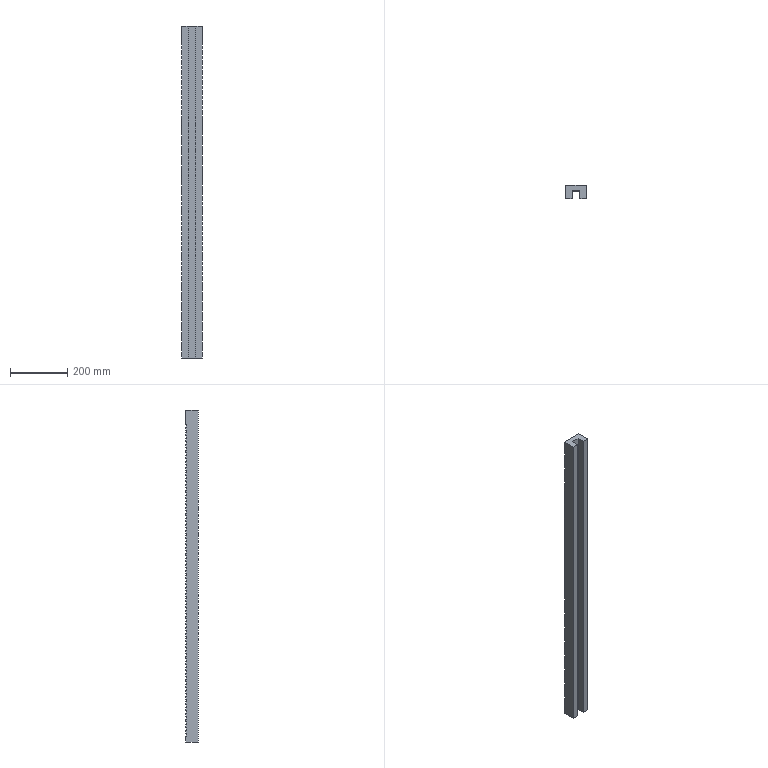Part | SolidWorks | features Extrusion 1, ICE 1, LPattern 1 | 1 solid | 230 faces | box 72 x 45 x 1160 mm | volume 2864880 mm3 | plane 230